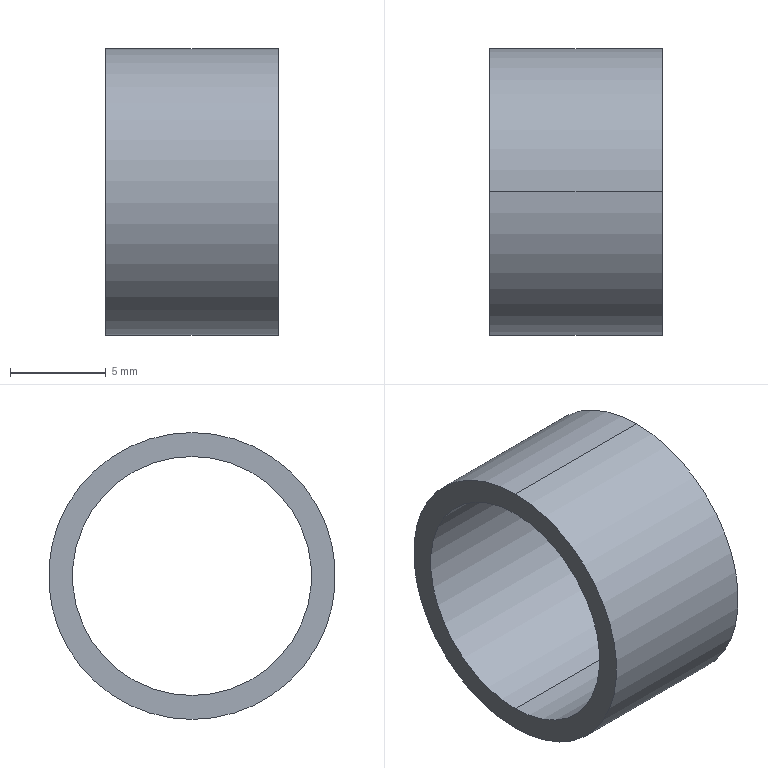Part | SolidWorks | features Revolution 1 | 1 solid | 6 faces | box 9 x 15 x 15 mm | volume 485.965 mm3 | cylinder 4 | plane 2 | commonest cylinder face diameters 12.5 x2 15 x2
STEP:
#1=CARTESIAN_POINT('',(9.,0.,7.5));
#2=VERTEX_POINT('',#1);
#3=CARTESIAN_POINT('',(9.,0.,-7.5));
#4=VERTEX_POINT('',#3);
#5=CARTESIAN_POINT('',(9.,0.,0.));
#6=DIRECTION('',(-1.,0.,0.));
#7=DIRECTION('',(0.,0.,1.));
#8=AXIS2_PLACEMENT_3D('',#5,#6,#7);
#9=CIRCLE('',#8,7.5);
#10=EDGE_CURVE('',#2,#4,#9,.T.);
#11=ORIENTED_EDGE('',*,*,#10,.T.);
#12=CARTESIAN_POINT('',(0.,0.,-7.5));
#13=VERTEX_POINT('',#12);
#14=CARTESIAN_POINT('',(0.,0.,-7.5));
#15=DIRECTION('',(-1.,0.,0.));
#16=VECTOR('',#15,1000.);
#17=LINE('',#14,#16);
#18=EDGE_CURVE('',#4,#13,#17,.T.);
#19=ORIENTED_EDGE('',*,*,#18,.T.);
#20=CARTESIAN_POINT('',(0.,0.,7.5));
#21=VERTEX_POINT('',#20);
#22=CARTESIAN_POINT('',(0.,0.,0.));
#23=DIRECTION('',(-1.,0.,0.));
#24=DIRECTION('',(0.,0.,1.));
#25=AXIS2_PLACEMENT_3D('',#22,#23,#24);
#26=CIRCLE('',#25,7.5);
#27=EDGE_CURVE('',#21,#13,#26,.T.);
#28=ORIENTED_EDGE('',*,*,#27,.F.);
#29=CARTESIAN_POINT('',(0.,0.,7.5));
#30=DIRECTION('',(-1.,0.,0.));
#31=VECTOR('',#30,1000.);
#32=LINE('',#29,#31);
#33=EDGE_CURVE('',#2,#21,#32,.T.);
#34=ORIENTED_EDGE('',*,*,#33,.F.);
#35=EDGE_LOOP('',(#11,#19,#28,#34));
#36=FACE_OUTER_BOUND('',#35,.T.);
#37=CARTESIAN_POINT('',(0.,0.,0.));
#38=DIRECTION('',(-1.,0.,0.));
#39=DIRECTION('',(0.,0.,1.));
#40=AXIS2_PLACEMENT_3D('',#37,#38,#39);
#41=CYLINDRICAL_SURFACE('',#40,7.5);
#42=ADVANCED_FACE('',(#36),#41,.T.);
#43=CARTESIAN_POINT('',(9.,0.,-6.25));
#44=VERTEX_POINT('',#43);
#45=CARTESIAN_POINT('',(9.,0.,6.25));
#46=VERTEX_POINT('',#45);
#47=CARTESIAN_POINT('',(9.,0.,0.));
#48=DIRECTION('',(-1.,0.,0.));
#49=DIRECTION('',(0.,0.,1.));
#50=AXIS2_PLACEMENT_3D('',#47,#48,#49);
#51=CIRCLE('',#50,6.25);
#52=EDGE_CURVE('',#44,#46,#51,.T.);
#53=ORIENTED_EDGE('',*,*,#52,.F.);
#54=CARTESIAN_POINT('',(0.,0.,-6.25));
#55=VERTEX_POINT('',#54);
#56=CARTESIAN_POINT('',(0.,0.,-6.25));
#57=DIRECTION('',(-1.,0.,0.));
#58=VECTOR('',#57,1000.);
#59=LINE('',#56,#58);
#60=EDGE_CURVE('',#44,#55,#59,.T.);
#61=ORIENTED_EDGE('',*,*,#60,.T.);
#62=CARTESIAN_POINT('',(0.,0.,6.25));
#63=VERTEX_POINT('',#62);
#64=CARTESIAN_POINT('',(0.,0.,0.));
#65=DIRECTION('',(-1.,0.,0.));
#66=DIRECTION('',(0.,0.,1.));
#67=AXIS2_PLACEMENT_3D('',#64,#65,#66);
#68=CIRCLE('',#67,6.25);
#69=EDGE_CURVE('',#55,#63,#68,.T.);
#70=ORIENTED_EDGE('',*,*,#69,.T.);
#71=CARTESIAN_POINT('',(0.,0.,6.25));
#72=DIRECTION('',(-1.,0.,0.));
#73=VECTOR('',#72,1000.);
#74=LINE('',#71,#73);
#75=EDGE_CURVE('',#46,#63,#74,.T.);
#76=ORIENTED_EDGE('',*,*,#75,.F.);
#77=EDGE_LOOP('',(#53,#61,#70,#76));
#78=FACE_OUTER_BOUND('',#77,.T.);
#79=CARTESIAN_POINT('',(0.,0.,0.));
#80=DIRECTION('',(-1.,0.,0.));
#81=DIRECTION('',(0.,0.,1.));
#82=AXIS2_PLACEMENT_3D('',#79,#80,#81);
#83=CYLINDRICAL_SURFACE('',#82,6.25);
#84=ADVANCED_FACE('',(#78),#83,.F.);
#85=CARTESIAN_POINT('',(0.,0.,0.));
#86=DIRECTION('',(-1.,0.,0.));
#87=DIRECTION('',(0.,0.,1.));
#88=AXIS2_PLACEMENT_3D('',#85,#86,#87);
#89=CIRCLE('',#88,6.25);
#90=EDGE_CURVE('',#63,#55,#89,.T.);
#91=ORIENTED_EDGE('',*,*,#90,.F.);
#92=ORIENTED_EDGE('',*,*,#69,.F.);
#93=EDGE_LOOP('',(#91,#92));
#94=FACE_BOUND('',#93,.T.);
#95=ORIENTED_EDGE('',*,*,#27,.T.);
#96=CARTESIAN_POINT('',(0.,0.,0.));
#97=DIRECTION('',(-1.,0.,0.));
#98=DIRECTION('',(0.,0.,1.));
#99=AXIS2_PLACEMENT_3D('',#96,#97,#98);
#100=CIRCLE('',#99,7.5);
#101=EDGE_CURVE('',#13,#21,#100,.T.);
#102=ORIENTED_EDGE('',*,*,#101,.T.);
#103=EDGE_LOOP('',(#95,#102));
#104=FACE_OUTER_BOUND('',#103,.T.);
#105=CARTESIAN_POINT('',(0.,7.5,0.));
#106=DIRECTION('',(1.,0.,0.));
#107=DIRECTION('',(0.,0.,-1.));
#108=AXIS2_PLACEMENT_3D('',#105,#106,#107);
#109=PLANE('',#108);
#110=ADVANCED_FACE('',(#94,#104),#109,.F.);
#111=ORIENTED_EDGE('',*,*,#60,.F.);
#112=CARTESIAN_POINT('',(9.,0.,0.));
#113=DIRECTION('',(-1.,0.,0.));
#114=DIRECTION('',(0.,0.,1.));
#115=AXIS2_PLACEMENT_3D('',#112,#113,#114);
#116=CIRCLE('',#115,6.25);
#117=EDGE_CURVE('',#46,#44,#116,.T.);
#118=ORIENTED_EDGE('',*,*,#117,.F.);
#119=ORIENTED_EDGE('',*,*,#75,.T.);
#120=ORIENTED_EDGE('',*,*,#90,.T.);
#121=EDGE_LOOP('',(#111,#118,#119,#120));
#122=FACE_OUTER_BOUND('',#121,.T.);
#123=CARTESIAN_POINT('',(0.,0.,0.));
#124=DIRECTION('',(-1.,0.,0.));
#125=DIRECTION('',(0.,0.,1.));
#126=AXIS2_PLACEMENT_3D('',#123,#124,#125);
#127=CYLINDRICAL_SURFACE('',#126,6.25);
#128=ADVANCED_FACE('',(#122),#127,.F.);
#129=ORIENTED_EDGE('',*,*,#10,.F.);
#130=CARTESIAN_POINT('',(9.,0.,0.));
#131=DIRECTION('',(-1.,0.,0.));
#132=DIRECTION('',(0.,0.,1.));
#133=AXIS2_PLACEMENT_3D('',#130,#131,#132);
#134=CIRCLE('',#133,7.5);
#135=EDGE_CURVE('',#4,#2,#134,.T.);
#136=ORIENTED_EDGE('',*,*,#135,.F.);
#137=EDGE_LOOP('',(#129,#136));
#138=FACE_OUTER_BOUND('',#137,.T.);
#139=ORIENTED_EDGE('',*,*,#117,.T.);
#140=ORIENTED_EDGE('',*,*,#52,.T.);
#141=EDGE_LOOP('',(#139,#140));
#142=FACE_BOUND('',#141,.T.);
#143=CARTESIAN_POINT('',(9.,7.5,0.));
#144=DIRECTION('',(-1.,0.,0.));
#145=DIRECTION('',(0.,0.,1.));
#146=AXIS2_PLACEMENT_3D('',#143,#144,#145);
#147=PLANE('',#146);
#148=ADVANCED_FACE('',(#138,#142),#147,.F.);
#149=ORIENTED_EDGE('',*,*,#18,.F.);
#150=ORIENTED_EDGE('',*,*,#135,.T.);
#151=ORIENTED_EDGE('',*,*,#33,.T.);
#152=ORIENTED_EDGE('',*,*,#101,.F.);
#153=EDGE_LOOP('',(#149,#150,#151,#152));
#154=FACE_OUTER_BOUND('',#153,.T.);
#155=CARTESIAN_POINT('',(0.,0.,0.));
#156=DIRECTION('',(-1.,0.,0.));
#157=DIRECTION('',(0.,0.,1.));
#158=AXIS2_PLACEMENT_3D('',#155,#156,#157);
#159=CYLINDRICAL_SURFACE('',#158,7.5);
#160=ADVANCED_FACE('',(#154),#159,.T.);
#161=CLOSED_SHELL('',(#42,#84,#110,#128,#148,#160));
#162=MANIFOLD_SOLID_BREP('',#161);
#163=CARTESIAN_POINT('',(0.,0.,0.));
#164=DIRECTION('',(0.,0.,1.));
#165=DIRECTION('',(1.,0.,0.));
#166=AXIS2_PLACEMENT_3D('',#163,#164,#165);
#167=(LENGTH_UNIT()NAMED_UNIT(*)SI_UNIT(.MILLI.,.METRE.));
#168=UNCERTAINTY_MEASURE_WITH_UNIT(LENGTH_MEASURE(0.00001),#167,'','');
#169=(NAMED_UNIT(*)PLANE_ANGLE_UNIT()SI_UNIT($,.RADIAN.));
#170=(NAMED_UNIT(*)SI_UNIT($,.STERADIAN.)SOLID_ANGLE_UNIT());
#171=(GEOMETRIC_REPRESENTATION_CONTEXT(3)GLOBAL_UNCERTAINTY_ASSIGNED_CONTEXT((#168))GLOBAL_UNIT_ASSIGNED_CONTEXT((#167,#169,#170))REPRESENTATION_CONTEXT('',''));
#172=ADVANCED_BREP_SHAPE_REPRESENTATION('',(#162,#166),#171);